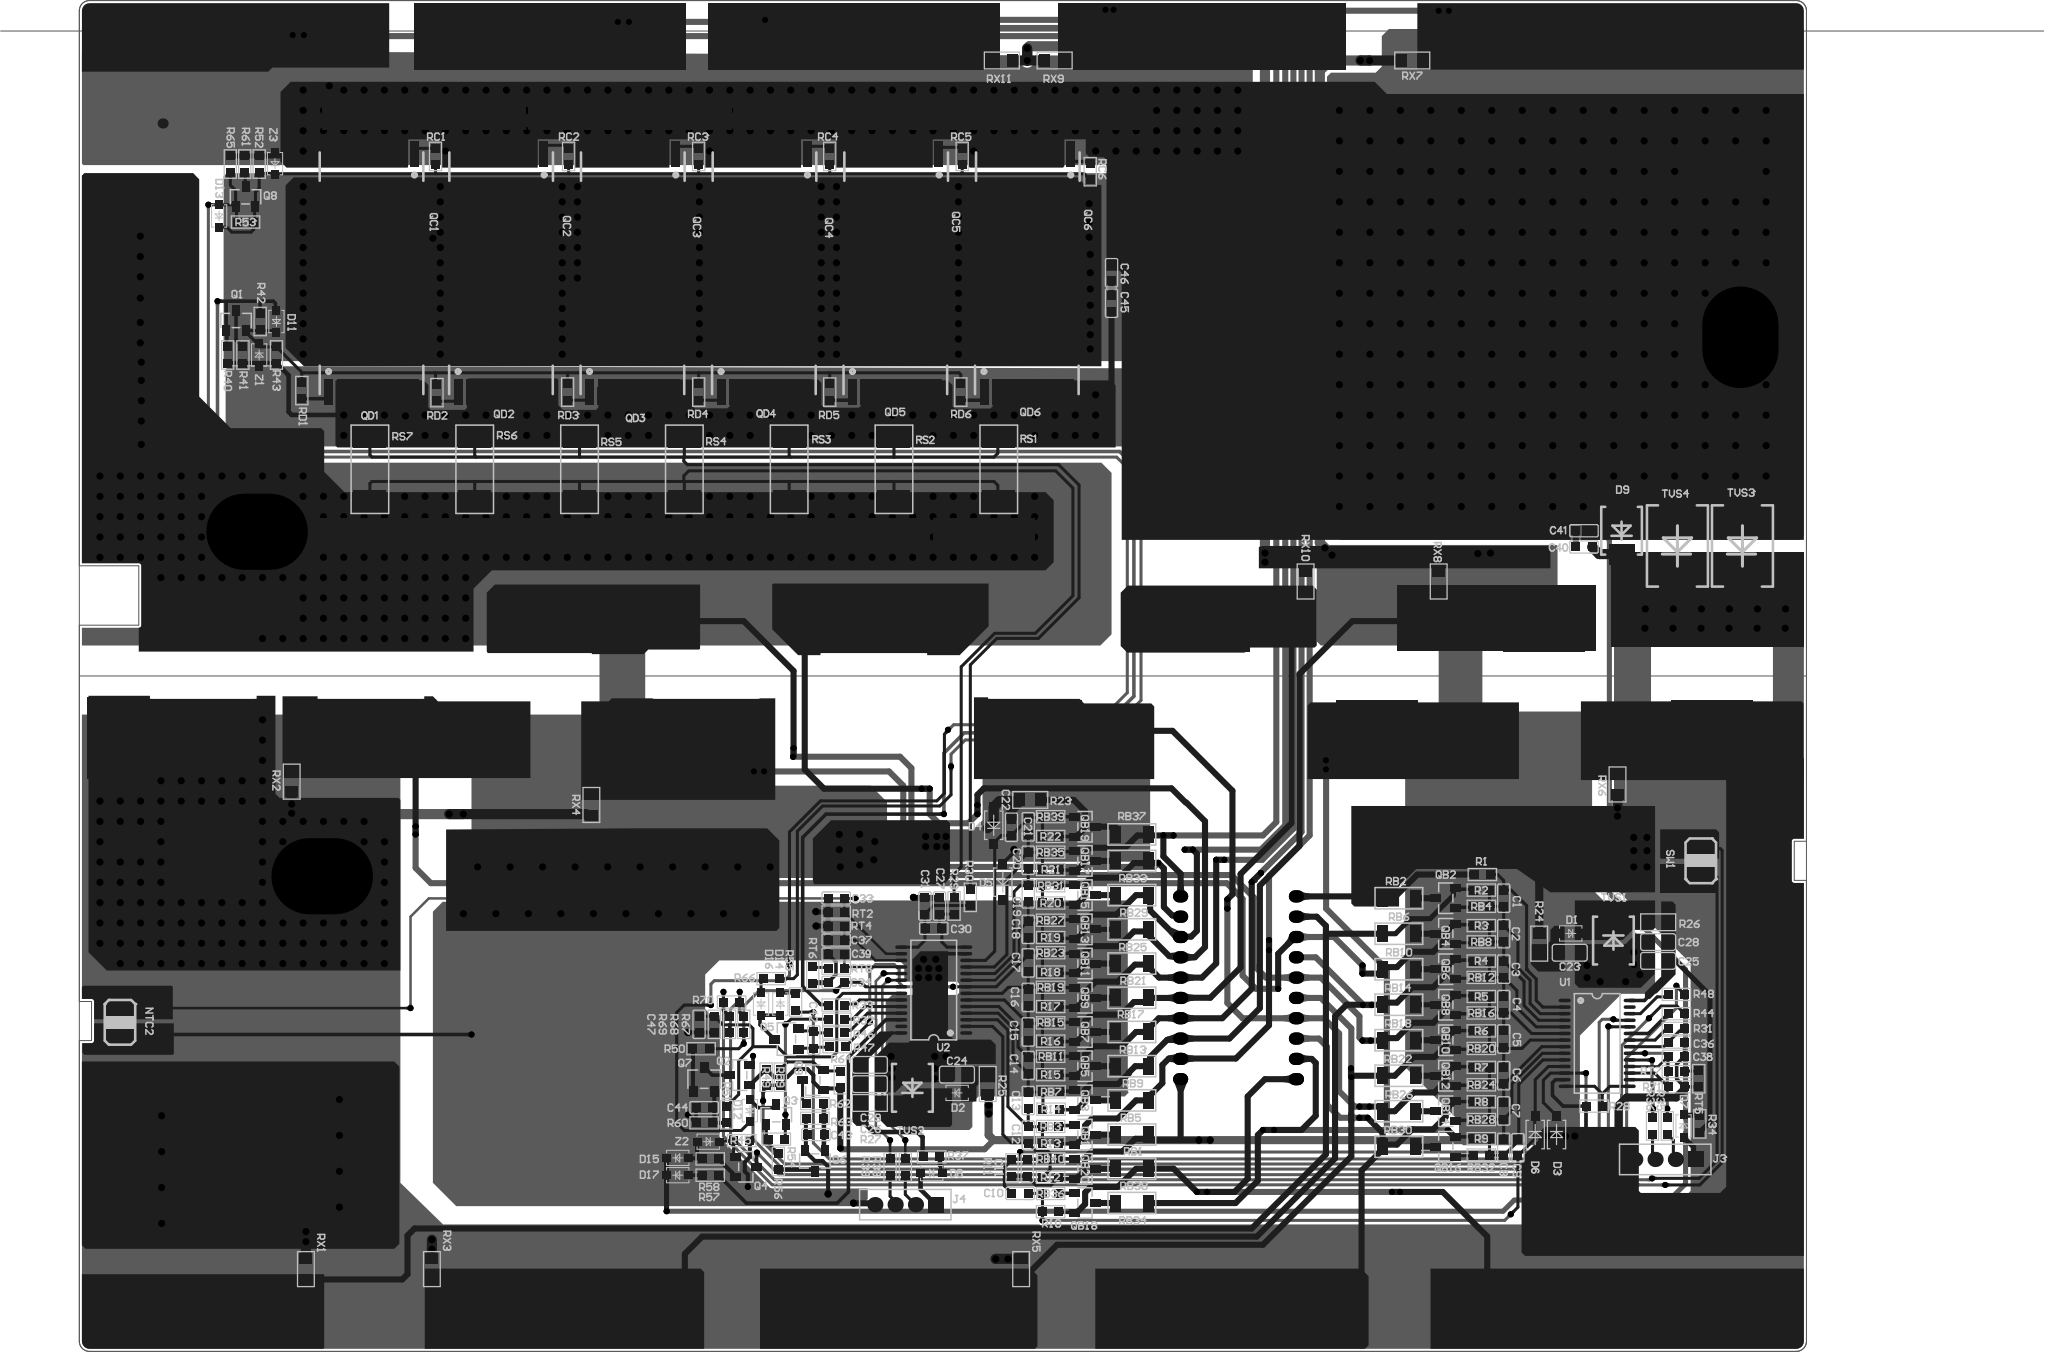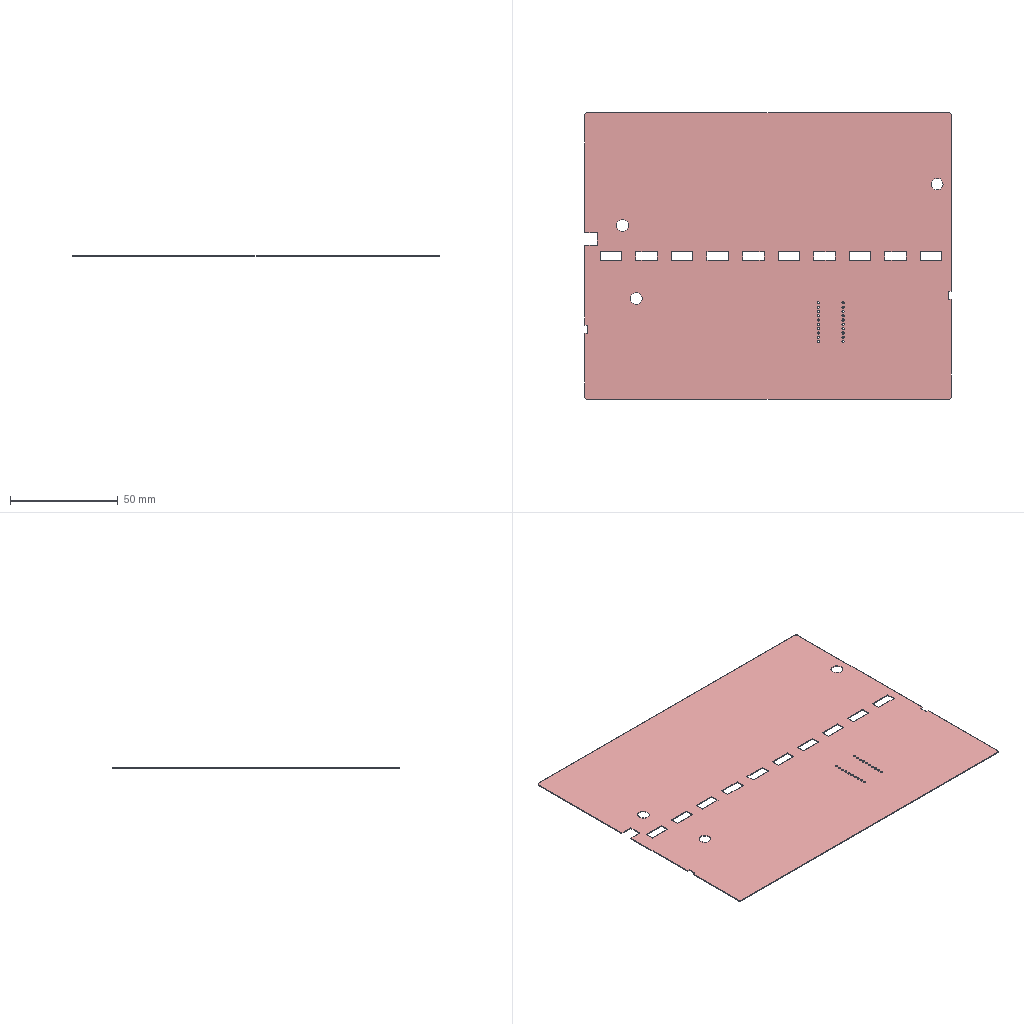Circuit board layout | Altium Designer | box 170 x 133 x 0.4 mm
Layer stack:
# Altium Designer layer stack of  (unit mm; dielectric type: 0 none, 1 core, 2 prepreg, 3 surface material)
index,name,kind,layer,copper_thickness_mm,dielectric_type,dielectric_thickness_mm,dielectric_material,dielectric_constant
0,Top Paste,other,,,,,,
1,Top Overlay,other,,,,,,
2,Top Solder,dielectric,,,3,0.0102,Solder Resist,3.5
3,Top Layer,copper,Top Layer,0.0356,,,,
4,Dielectric 1,dielectric,,,0,0.32,FR-4,4.8
5,Bottom Layer,copper,Bottom Layer,0.0356,,,,
6,Bottom Solder,dielectric,,,3,0.0102,Solder Resist,3.5
7,Bottom Overlay,other,,,,,,
8,Bottom Paste,other,,,,,,
# drill layer pairs: low layer,high layer
drill_pair,Top Layer,Bottom Layer
Part placement:
Designator,Comment,Layer,Footprint,Center-X(mm),Center-Y(mm),Rotation
RS7,R010,TopLayer,R2512L,28.6,85.85,90
RS6,R010,TopLayer,R2512L,38.917,85.85,90
RD6,47R,TopLayer,R0603A,86.76,93.45,90
RD5,47R,TopLayer,R0603A,73.86,93.45,90
RC6,47R,TopLayer,R0603A,99.5,115.15,90
RC5,47R,TopLayer,R0603A,86.9,116.65,90
QD6,N MOS*,TopLayer,TOLL_123,93.26,96.8,0
QD5,N MOS*,TopLayer,TOLL_123,80.32,96.8,0
QC6,N MOS*,TopLayer,TOLL_123,93.36,113.5,180
QC5,N MOS*,TopLayer,TOLL_123,80.4,113.5,180
R71,10K,TopLayer,R0603A,157.2,25.05,180
R70,100K,TopLayer,R0603A,64.2,33.4,0
R69,10M,TopLayer,R0603A,62.5,31.2,270
R68,100K,TopLayer,R0603A,64,31.2,90
R67,100K,TopLayer,R0603A,65.4,31.2,270
C47,1nF25V,TopLayer,C0603A,61,31.2,90
SW1,SW_1,TopLayer,RT2.3X1.2-2,159.6,47.3,90
TVS4,SMBJ75A*,TopLayer,SMC_MDO-214AB),157.3,78.3,270
TVS3,SMBJ75A*,TopLayer,SMC_MDO-214AB),163.7,78.3,270
RB40,510R,TopLayer,R0603A,95.6,17.95,180
RB39,510R,TopLayer,R0603A,95.6,51.65,180
RB38,100R,TopLayer,R1206A,103.6,16.977,180
RB37,100R,TopLayer,R1206A,103.6,49.9,180
RB36,510R,TopLayer,R0603A,95.6,14.55,180
RB35,510R,TopLayer,R0603A,95.6,48.15,180
RB34,100R,TopLayer,R1206A,103.6,13.609,180
RB33,100R,TopLayer,R1206A,103.6,47.291,180
RB32,510R,TopLayer,R0603A,138,18.332,0
RB31,510R,TopLayer,R0603A,95.6,44.85,180
RB30,100R,TopLayer,R1206A,129.884,19.15,0
RB29,100R,TopLayer,R1206A,103.6,43.923,180
RB28,510R,TopLayer,R0603A,138,21.83,0
RB27,510R,TopLayer,R0603A,95.6,41.45,180
RB26,100R,TopLayer,R1206A,129.884,22.645,0
RB25,100R,TopLayer,R1206A,103.6,40.555,180
RB24,510R,TopLayer,R0603A,138,25.25,0
RB23,510R,TopLayer,R0603A,95.6,38.25,180
RB22,100R,TopLayer,R1206A,129.884,26.141,0
RB21,100R,TopLayer,R1206A,103.6,37.186,180
RB20,510R,TopLayer,R0603A,138,28.826,0
RB19,510R,TopLayer,R0603A,95.6,34.85,180
RB18,100R,TopLayer,R1206A,129.884,29.636,0
RB17,100R,TopLayer,R1206A,103.6,33.818,180
RB16,510R,TopLayer,R0603A,138,32.324,0
RB15,510R,TopLayer,R0603A,95.6,31.35,180
RB14,100R,TopLayer,R1206A,129.884,33.131,0
RB13,100R,TopLayer,R1206A,103.6,30.45,180
RB12,510R,TopLayer,R0603A,138,35.822,0
RB11,510R,TopLayer,R0603A,95.6,28.05,180
RB10,100R,TopLayer,R1206A,129.884,36.627,0
RB9,100R,TopLayer,R1206A,103.6,27.082,180
RB8,510R,TopLayer,R0603A,138,39.32,0
RB7,510R,TopLayer,R0603A,95.65,24.55,180
RB6,100R,TopLayer,R1206A,129.884,40.122,0
RB5,100R,TopLayer,R1206A,103.6,23.714,180
RB4,510R,TopLayer,R0603A,138,42.818,0
RB3,510R,TopLayer,R0603A,95.6,21.15,180
RB2,100R,TopLayer,R1206A,129.884,43.617,0
RB1,100R,TopLayer,R1206A,103.6,20.346,180
QB20,MMBT5551,TopLayer,SOT23-3,98.992,16.977,270
QB19,MMBT5551,TopLayer,SOT23-3,98.992,50.659,270
QB18,MMBT5551,TopLayer,SOT23-3,98.992,13.609,270
QB17,MMBT5551,TopLayer,SOT23-3,98.992,47.291,270
QB16,MMBT5551,TopLayer,SOT23-3,134.492,19.15,90
QB15,MMBT5551,TopLayer,SOT23-3,98.992,43.923,270
QB14,MMBT5551,TopLayer,SOT23-3,134.492,22.645,90
QB13,MMBT5551,TopLayer,SOT23-3,98.992,40.555,270
QB12,MMBT5551,TopLayer,SOT23-3,134.492,26.141,90
QB11,MMBT5551,TopLayer,SOT23-3,98.992,37.186,270
QB10,MMBT5551,TopLayer,SOT23-3,134.492,29.636,90
QB9,MMBT5551,TopLayer,SOT23-3,98.992,33.818,270
QB8,MMBT5551,TopLayer,SOT23-3,134.492,33.131,90
QB7,MMBT5551,TopLayer,SOT23-3,98.992,30.45,270
QB6,MMBT5551,TopLayer,SOT23-3,134.492,36.627,90
QB5,MMBT5551,TopLayer,SOT23-3,98.992,27.082,270
QB4,MMBT5551,TopLayer,SOT23-3,134.492,40.122,90
QB3,MMBT5551,TopLayer,SOT23-3,98.992,23.714,270
QB2,MMBT5551,TopLayer,SOT23-3,134.492,43.617,90
QB1,MMBT5551,TopLayer,SOT23-3,98.992,20.346,270
R49,1M,TopLayer,R0603A,67.6,26,90
NTC2,10K B=3435,TopLayer,RT2.3X1.2-2,4,31.4,270
C46,0.1uF100V,TopLayer,C0603A,101.6,105.2,270
C45,0.1uF100V,TopLayer,C0603A,101.6,102.2,270
D7,BAV21W,TopLayer,SOD323A,157.9,21.2,270
RX11,0R,TopLayer,R0805L,90.8,126.1,180
RX3,0R,TopLayer,R0805L,34.7,7.1,270
Q9,MMBT5401,TopLayer,SOT23-3,72.192,25.7,90
R64,1M,TopLayer,R0603A,74.9,25.75,270
Q8,MMBT5401,TopLayer,SOT23-3,16.36,112.684,0
R36,100R,TopLayer,R0603A,154.85,21.2,270
R35,100R,TopLayer,R0603A,156.3,21.2,270
R38,100R,TopLayer,R0603A,81.3,17.15,270
R37,100R,TopLayer,R0603A,83.9,18.15,0
RD4,47R,TopLayer,R0603A,60.96,93.45,90
RD3,47R,TopLayer,R0603A,48.06,93.45,270
RD2,47R,TopLayer,R0603A,35.2,93.4,270
TVS2,SMBJ64A,TopLayer,SMB_A,82,24.95,90
TVS1,SMBJ64A,TopLayer,SMB_A,151,39.45,270
D4,BAT46W,TopLayer,SOD123,90,50.8,90
D3,BAT46W,TopLayer,SOD123,145.4,20.35,270
R61,510R,TopLayer,R0603A,16.28,115.9,90
R33,1K,TopLayer,R0603A,74.5,33.1,180
C26,1uF100V,TopLayer,C0805L,77.81,25.31,180
C25,1uF100V,TopLayer,C0805L,155.4,37.45,0
C24,1uF100V,TopLayer,C0805L,86.384,26.25,0
C23,1uF100V,TopLayer,C0805L,146.7,38.25,180
C22,1uF50V,TopLayer,C0603A,91.75,50.6,270
C21,0.1uF50V,TopLayer,C0603A,93.4,50.65,270
C20,0.1uF50V,TopLayer,C0603A,93.4,47.35,270
C19,0.1uF50V,TopLayer,C0603A,93.4,44.05,270
C17,0.1uF50V,TopLayer,C0603A,93.4,37.25,270
C16,0.1uF50V,TopLayer,C0603A,93.4,33.85,270
C15,0.1uF50V,TopLayer,C0603A,93.4,30.45,270
C14,0.1uF50V,TopLayer,C0603A,93.4,27.15,270
C13,0.1uF50V,TopLayer,C0603A,93.4,23.7,270
C12,0.1uF50V,TopLayer,C0603A,93.4,20.3,270
C8,0.1uF50V,TopLayer,C0603A,140.2,19.082,90
C7,0.1uF50V,TopLayer,C0603A,140.2,22.673,90
C6,0.1uF50V,TopLayer,C0603A,140.2,26.15,90
C5,0.1uF50V,TopLayer,C0603A,140.2,29.755,90
C4,0.1uF50V,TopLayer,C0603A,140.2,33.145,90
C3,0.1uF50V,TopLayer,C0603A,140.2,36.636,90
C1,0.1uF50V,TopLayer,C0603A,140.2,43.617,90
RT2,10K B=3435,TopLayer,R0603A,74.5,42.26,180
R66,1M,TopLayer,R0603A,68.1,35.7,180
R65,5.1M,TopLayer,R0603A,14.86,115.9,90
R63,1M,TopLayer,R0603A,72.4,21.95,180
R62,3M,TopLayer,R0603A,72.4,23.4,180
R59,3M,TopLayer,R0603A,69,26,270
R58,1M,TopLayer,R0603A,62.1,17.95,0
R57,3M,TopLayer,R0603A,62.1,16.35,0
R56,3M,TopLayer,R0603A,68.8,17.7,270
R55,1M,TopLayer,R0603A,70.5,33.4,270
R54,1M,TopLayer,R0603A,68.6,19.9,0
R53,0R/NC*,TopLayer,R0603A,16.36,110.192,0
R52,5.1M,TopLayer,R0603A,17.7,115.9,90
R51,100K,TopLayer,R0603A,63.7,22.3,90
R50,100K,TopLayer,R0603A,61.2,28.8,0
RC1,47R,TopLayer,R0603A,35.06,116.65,90
R48,10M,TopLayer,R0603A,157.2,34.15,180
R47,10K,TopLayer,R0603A,74.6,29,0
R46,10K,TopLayer,R0603A,74.56,30.36,0
R45,510K,TopLayer,R0603A,65.2,19.75,180
R44,1M,TopLayer,R0603A,157.2,32.25,180
R43,5.1M,TopLayer,R0603A,19.4,97.1,270
R42,0R/NC*,TopLayer,R0603A,17.8,100.4,270
R41,510R,TopLayer,R0603A,16.1,97.1,270
R40,5.1M,TopLayer,R0603A,14.6,97.1,270
R39,100R,TopLayer,R0603A,79.8,17.15,270
R34,100R,TopLayer,R0603A,159.5,21.4,90
R32,1K,TopLayer,R0603A,74.56,31.71,180
R31,1K,TopLayer,R0603A,157.2,30.8,180
R30,10R,TopLayer,R0603A,87.7,43.7,90
R29,10R,TopLayer,R0603A,86.1,42.85,270
R28,1K,TopLayer,R0603A,149.1,23.15,0
R27,100R,TopLayer,R0805L,77.81,23.46,0
R26,100R,TopLayer,R0805L,155.4,41.25,180
R25,1K,TopLayer,R0805L,89.41,25.326,270
R20,510R,TopLayer,R0603A,95.6,43.15,180
R19,510R,TopLayer,R0603A,95.6,39.75,180
R18,510R,TopLayer,R0603A,95.6,36.35,180
R17,510R,TopLayer,R0603A,95.6,32.95,180
R16,510R,TopLayer,R0603A,95.6,29.55,180
R15,510R,TopLayer,R0603A,95.6,26.25,180
R14,510R,TopLayer,R0603A,95.65,22.85,180
R13,510R,TopLayer,R0603A,95.6,19.5,180
R12,510R,TopLayer,R0603A,95.6,16.15,180
R11,510R,TopLayer,R0603A,91.8,17.05,90
R10,510R,TopLayer,R0603A,95.6,12.75,180
R8,510R,TopLayer,R0603A,138,23.573,0
R7,510R,TopLayer,R0603A,138,26.964,0
R6,510R,TopLayer,R0603A,138,30.555,0
R5,510R,TopLayer,R0603A,138,33.945,0
R4,510R,TopLayer,R0603A,138,37.436,0
R3,510R,TopLayer,R0603A,138,40.927,0
R1,510R,TopLayer,R0603A,138.1,45.95,0
Q5,AM2394,TopLayer,SOT23-3L,69.6,29.75,90
Q2,MMBT5401,TopLayer,SOT23-3,64.992,26.2,90
Q1,MMBT5401,TopLayer,SOT23-3,15.425,100.508,0
D11,BAV21W,TopLayer,SOD323A,19.4,100.4,90
D9,RS3M,TopLayer,SMB_A,151.8,79.8,90
D2,BAV21W,TopLayer,SOD323A,86.4,24.45,0
D1,BAV21W,TopLayer,SOD323A,146.8,40.15,180
C44,1nF25V,TopLayer,C0603A,61.5,23,180
C37,1nF25V,TopLayer,C0603A,74.5,39.5,180
C36,1uF25V,TopLayer,C0603A,157.2,29.45,180
C34,1uF25V,TopLayer,C0603A,74.5,35.34,0
C33,1nF25V,TopLayer,C0603A,74.5,43.64,180
C31,1uF25V,TopLayer,C0603A,83.233,42.85,270
C30,1nF25V,TopLayer,C0603A,84.1,40.65,0
C29,0.1uF100V,TopLayer,C0805L,77.81,27.21,180
C28,0.1uF100V,TopLayer,C0805L,155.4,39.3,0
C27,1uF25V,TopLayer,C0603A,84.667,42.85,90
C18,0.1uF50V,TopLayer,C0603A,93.4,40.55,270
C11,1uF50V,TopLayer,C0603A,93.3,17.05,90
C10,0.1uF50V,TopLayer,C0603A,92.6,14.55,0
QC4,N MOS*,TopLayer,TOLL_123,67.44,113.5,180
QC3,N MOS*,TopLayer,TOLL_123,54.48,113.5,180
Z3,15V,TopLayer,SOD323A,19.26,115.942,90
Z2,3.3V,TopLayer,SOD323A,61.9,19.65,180
Z1,15V,TopLayer,SOD323A,17.7,97.1,270
RX10,0R,TopLayer,R0805L,120.7,74.8,270
RX9,0R,TopLayer,R0805L,96,126.1,0
RX8,0R,TopLayer,R0805L,133.8,74.8,270
RX7,0R,TopLayer,R0805L,131.2,126.1,0
RX6,0R,TopLayer,R0805L,151.4,54.816,270
RX5,0R,TopLayer,R0805L,92.7,7.1,270
RX4,0R,TopLayer,R0805L,50.4,52.8,90
RX2,0R,TopLayer,R0805L,20.9,55.1,90
RX1,0R,TopLayer,R0805L,22.3,7.1,270
RT8,0R,TopLayer,R0603A,74.5,36.74,0
RT7,0R,TopLayer,R0603A,157.2,26.55,180
RT6,10K B=3435,TopLayer,R0603A,72.19,36.07,270
RT5,10K B=3435,TopLayer,R0603A,159.4,25.85,270
RT4,10K B=3435,TopLayer,R0603A,74.5,40.88,180
RS5,R010,TopLayer,R2512L,49.233,85.85,90
RS4,R010,TopLayer,R2512L,59.55,85.85,90
RD1,47R,TopLayer,R0603A,21.9,93.6,270
RC4,47R,TopLayer,R0603A,73.86,116.65,90
RC3,47R,TopLayer,R0603A,60.96,116.65,270
RC2,47R,TopLayer,R0603A,48.16,116.65,270
R60,10M,TopLayer,R0603A,61.5,21.5,0
R24,1K,TopLayer,R0805L,143.7,39.15,90
R23,510R,TopLayer,R0805L,93.6,53.3,0
R22,510R,TopLayer,R0603A,95.6,49.7,180
R21,510R,TopLayer,R0603A,95.6,46.45,180
R9,510R,TopLayer,R0603A,138,19.95,0
R2,510R,TopLayer,R0603A,138,44.417,0
QC2,N MOS*,TopLayer,TOLL_123,41.52,113.5,180
QC1,N MOS*,TopLayer,TOLL_123,28.76,113.5,180
QD2,N MOS*,TopLayer,TOLL_123,41.5,96.8,0
Q7,AM2394,TopLayer,SOT23-3L,61.5,25.8,0
Q6,MMBT5551,TopLayer,SOT23-3,72.4,17.742,180
Q4,MMBT5551,TopLayer,SOT23-3,65.608,17.175,270
Q3,MMBT5401,TopLayer,SOT23-3,68.6,22.308,0
J4,CH-2.0-4P,TopLayer,Test2.0-4P,81.3,13.45,180
J3,CH-2.0-4P,TopLayer,Test2.0-4P,156.1,17.9,180
D17,BAV21W,TopLayer,SOD323A,58.9,16.35,0
D16,BAV21W,TopLayer,SOD323A,67.1,33.2,90
D15,BAV21W,TopLayer,SOD323A,58.9,18.05,0
D14,BAV21W,TopLayer,SOD323A,69,33.2,270
D13,BAV21W,TopLayer,SOD323A,13.76,110.792,90
D12,BAV21W,TopLayer,SOD323A,66,22.7,90
C43,0.1uF50V,TopLayer,C0603A,72.5,20.35,0
C42,10nF25V,TopLayer,C0603A,72.3,29.65,90
C9,0.1uF50V,TopLayer,C0603A,141.6,19.05,90
C2,0.1uF50V,TopLayer,C0603A,140.2,40.127,90
D6,BAT46W,TopLayer,SOD123,143.3,20.35,270
C38,1nF25V,TopLayer,C0603A,157.2,28.05,0
RS3,R010,TopLayer,R2512L,69.867,85.85,90
QD4,N MOS*,TopLayer,TOLL_123,67.38,96.8,0
U2,SH3676010,TopLayer,TSSOP-28L(PIN间距0.65mm),84.1,34.575,180
U1,SH3676010,TopLayer,TSSOP-28L(PIN间距0.65mm),149.4,29.325,0
RS2,R010,TopLayer,R2512L,80.183,85.85,90
RS1,R010,TopLayer,R2512L,90.5,85.85,90
QD3,N MOS*,TopLayer,TOLL_123,54.44,96.8,0
D8,BAV21W,TopLayer,SOD323A,83.9,16.55,180
D5,BAT46W,TopLayer,SOD123,90.9,45.2,90
C41,0.1uF50V,TopLayer,C0603A,148.1,79.8,180
C39,1nF25V,TopLayer,C0603A,74.5,38.12,180
C40,0.1uF50V,TopLayer,C0603A,148.1,78.2,0
QD1,N MOS*,TopLayer,TOLL_123,28.76,96.8,0
Pad and via stacks:
# Altium Designer via and pad stacks of  (unit mm). Each distinct definition once, with the count of objects using it.
# via: kind,start_layer,end_layer,hole_mm,diameter_mm,mode(0 simple;1 top-mid-bottom;2 full stack),diameter_per_layer,count,example_net
# pad: kind,layer,hole_mm,hole_type(0 round;1 square;2 slot),plating,top_size,top_shape(1 round;2 rect;3 octagon;9 rounded rect),mid_size,bottom_size,mode,footprint,size_per_layer,count,example
pad,Top Layer,0,0,plated,8x6,2,8x6,8x6,0,,,21,81
pad,Top Layer,0,0,plated,3x3,1,3x3,3x3,0,,,23,86
pad,Top Layer,0,0,plated,2.5x20,2,2.5x20,2.5x20,0,,,7,82
pad,Top Layer,0,0,plated,2.5x10,2,2.5x10,2.5x10,0,,,1,83
pad,Top Layer,0,0,plated,0.8x0.8,2,0.8x0.8,0.8x0.8,0,R0603A,,208,R9.1
pad,Top Layer,0,0,plated,0.8x0.8,2,0.8x0.8,0.8x0.8,0,C0603A,,78,C9.1
pad,Top Layer,0,0,plated,0.9x0.8,2,0.9x0.8,0.9x0.8,0,SOD123,,8,D6.2
pad,Top Layer,0,0,plated,1.016x1.27,2,1.016x1.27,1.016x1.27,0,R0805L,,32,R24.1
pad,Top Layer,0,0,plated,1.5x1.5,2,1.5x1.5,1.5x1.5,0,Test2.0-4P,,2,J3.1
pad,Top Layer,0,0,plated,1.5x1.5,1,1.5x1.5,1.5x1.5,0,Test2.0-4P,,6,J3.2
pad,Top Layer,0,2,plated,1.2x0.35,1,1.2x0.35,1.2x0.35,0,TSSOP-28L(PIN\u00BC\u00E4\u00BE\u00E00.65mm),,56,U1.1
pad,Top Layer,0,0,plated,0.7x1,2,0.7x1,0.7x1,0,SOT23-3,,81,QB16.1
pad,Top Layer,0,0,plated,1x1.6,2,1x1.6,1x1.6,0,R1206A,,40,RB10.1
pad,Top Layer,0,0,plated,1.016x1.27,2,1.016x1.27,1.016x1.27,0,C0805L,,12,C23.2
pad,Top Layer,0,0,plated,0.8x0.7,2,0.8x0.7,0.8x0.7,0,SOD323A,,28,D1.1
pad,Top Layer,0,0,plated,2x2.5,2,2x2.5,2x2.5,0,SMB A,,6,TVS1.1
pad,Top Layer,0,0,plated,0.8x1,2,0.8x1,0.8x1,0,SOT23-3L,,6,Q7.1
pad,Top Layer,0,0,plated,2.5x0.8,2,2.5x0.8,2.5x0.8,0,TOLL_123,,12,QC3.1
pad,Top Layer,0,0,plated,1.7x0.8,2,1.7x0.8,1.7x0.8,0,TOLL_123,,84,QC3.2
pad,Top Layer,0,0,plated,0.8x8,2,0.8x8,0.8x8,0,TOLL_123,,12,QC3.2
pad,Top Layer,0,0,plated,9.9x8,2,9.9x8,9.9x8,0,TOLL_123,,12,QC3.3
pad,Top Layer,0,0,plated,2x3.2,2,2x3.2,2x3.2,0,R2512L,,14,RS6.2
pad,Top Layer,0,0,plated,1.8x3.2,2,1.8x3.2,1.8x3.2,0,SMC_MDO-214AB),,4,TVS3.2
pad,Top Layer,0,0,plated,9x6,2,9x6,9x6,0,,,1,81
pad,Top Layer,0,0,plated,1.2x2.3,1,1.2x2.3,1.2x2.3,0,RT2.3X1.2-2,,4,SW1.1
pad,Top Layer,0,0,plated,1x1,1,1x1,1x1,0,,,2,75
pad,Multi-Layer,1,0,plated,1.5x1.2,1,1.5x1.2,1.5x1.2,0,,,20,
pad,Multi-Layer,5.5,0,plated,7.5x10,1,7.5x10,7.5x10,0,,,3,66
via,Top Layer,Bottom Layer,0.4,0.6,0,,99,B15
via,Top Layer,Bottom Layer,0.5,0.7,0,,953,GND
Copper pours:
name,layer,net,type(0 solid;1 hatched;2 none)
NONET_L02_P-001,Top Layer,NetR68_2,0
NONET_L02_P-001,Top Layer,NetR67_1,0
NONET_L02_P-001,Top Layer,P-/C-,0
NONET_L02_P-001,Top Layer,B4,0
NONET_L02_P-001,Top Layer,B14,0
NONET_L02_P-001,Top Layer,B13,0
NONET_L02_P-001,Top Layer,B+,0
NONET_L02_P-001,Top Layer,B17,0
NONET_L02_P-001,Top Layer,B+,0
NONET_L02_P-001,Top Layer,B10,0
NONET_L02_P-001,Top Layer,GND,0
NONET_L02_P-001,Top Layer,B12,0
NONET_L02_P-001,Top Layer,NetC33_1,0
NONET_L02_P-001,Top Layer,GND,0
NONET_L02_P-001,Top Layer,GND,0
NONET_L02_P-001,Top Layer,B10,0
NONET_L02_P-001,Top Layer,VBAT_S,0
NONET_L02_P-001,Top Layer,B10,0
NONET_L02_P-001,Top Layer,NetD1_1,0
NONET_L02_P-001,Top Layer,NetC23_2,0
NONET_L02_P-001,Top Layer,B6,0
NONET_L02_P-001,Top Layer,VBAT_M,0
NONET_L02_P-001,Top Layer,NetC24_2,0
NONET_L02_P-001,Top Layer,GND,0
NONET_L02_P-001,Top Layer,NetD2_1,0
NONET_L02_P-001,Top Layer,GND,0
NONET_L02_P-001,Top Layer,NetC45_2,0
NONET_L02_P-001,Top Layer,B+,0
NONET_L02_P-001,Top Layer,B9,0
NONET_L02_P-001,Top Layer,B+,0
NONET_L02_P-001,Top Layer,B8,0
NONET_L02_P-001,Top Layer,B10,0
NONET_L02_P-001,Top Layer,B16,0
NONET_L02_P-001,Top Layer,B2,0
NONET_L02_P-001,Top Layer,B18,0
NONET_L02_P-001,Top Layer,B11,0
NONET_L02_P-001,Top Layer,B15,0
NONET_L02_P-001,Top Layer,B19,0
NONET_L02_P-001,Top Layer,B7,0
NONET_L02_P-001,Top Layer,B5,0
NONET_L02_P-001,Top Layer,B3,0
NONET_L02_P-001,Top Layer,B1,0
NONET_L02_P-001,Top Layer,MSO_D-,0
NONET_L02_P-001,Bottom Layer,GND,0
NONET_L02_P-001,Bottom Layer,B+,0
NONET_L02_P-001,Bottom Layer,GND,0
NONET_L02_P-001,Bottom Layer,GND,0
NONET_L02_P-001,Bottom Layer,B10,0
NONET_L02_P-001,Bottom Layer,P-/C-,0
NONET_L02_P-001,Bottom Layer,P-/C-,0
NONET_L02_P-001,Bottom Layer,MSO_D-,0
NONET_L02_P-001,Bottom Layer,NetC45_2,0
NONET_L02_P-001,Bottom Layer,GND,0
Design rules, without the lines most boards share:
# Altium Designer design rules of  (exported by Altium Designer, unit mm)
# columns: name | kind | enabled | priority | scope1 | scope2 | descriptor | typed fields (field=value)
Schematic Supply Nets_3 | 41 | enabled | 1 | InNet('B0') | All | Supply Net(s)(InNet('B0')) |
Schematic Supply Nets_2 | 41 | enabled | 2 | InNet('P-/C-') | All | Supply Net(s)(InNet('P-/C-')) |
Schematic Supply Nets_1 | 41 | enabled | 3 | InNet('GND') | All | Supply Net(s)(InNet('GND')) |
Schematic Supply Nets | 41 | enabled | 4 | InNet('B10') | All | Supply Net(s)(InNet('B10')) |
NetAntennae | 56 | enabled | 1 | All | All | Net Antennae (Tolerance=0mm) (All) |
SilkToSilkClearance | 55 | enabled | 1 | All | All | Silk to Silk (Clearance=0.254mm) (All),(All) |
SilkToSolderMaskClearance | 54 | enabled | 1 | IsPad | All | Silk To Solder Mask (Clearance=0.254mm) (IsPad),(All) |
MinimumSolderMaskSliver | 53 | enabled | 1 | All | All | Minimum Solder Mask Sliver (Gap=0.254mm) (All),(All) |
HoleToHoleClearance | 52 | enabled | 1 | All | All | Hole To Hole Clearance (Gap=0.254mm) (All),(All) | gap=0.254
DiffPairsRouting | 51 | enabled | 1 | All | All | Differential Pairs Uncoupled Length using the Gap Constraints (Min=0.254mm) (Max=0.254mm) (Prefered=0.254mm)  and Width Constraints (Min=0.381mm) (Max=0.381mm) (Prefered=0.381mm) (All) |
HoleSize | 42 | enabled | 1 | All | All | Hole Size Constraint (Min=0.025mm) (Max=50mm) (All) |
Height | 50 | enabled | 1 | All | All | Height Constraint (Min=0mm) (Max=25.4mm) (Prefered=12.7mm) (All) | min_height=0 max_height=25.4
ComponentClearance | 24 | enabled | 1 | All | All | Component Clearance Constraint ( Horizontal Gap = 0.2mm, Vertical Gap = 0.2mm ) (All),(All)  | gap=0.2
SolderMaskExpansion | 13 | enabled | 1 | All | All | Solder Mask Expansion (Expansion =0.102mm) (All) | expansion=0.1016
PasteMaskExpansion | 14 | enabled | 1 | All | All | Paste Mask Expansion (Expansion =0mm) (All) | expansion=0
RoutingVias | 11 | enabled | 1 | All | All | Routing Via (MinHoleWidth=0.4mm) (MaxHoleWidth=0.5mm) (PreferredHoleWidth=0.4mm) (MinWidth=0.6mm) (MaxWidth=7mm) (PreferedWidth=0.6mm) (All) | via_min_hole=0.4 via_max_hole=0.5 via_preferred_diameter=0.6 via_preferred_hole=0.4
RoutingCorners | 10 | enabled | 1 | All | All | Routing Corners (Style=45-Degree) (Min Setback=2.54mm) (Max Setback=2.54mm) (All) |
Width | 2 | enabled | 1 | All | All | Width Constraint (Min=0.2mm) (Max=2mm) (Preferred=0.25mm) (All) |
PolygonConnect | 20 | enabled | 1 | All | All | Polygon Connect Rule(Direct Connect )(Conductor Width=0.254mm) (Relief Angle=90 Angle) (Entries=4) (Air Gap Width=0.254mm) (All),(All) | connect_style(0=relief,1=direct,2=none)=1 relief_conductor_width=0.254 relief_entries=4
PlaneClearance | 12 | enabled | 1 | All | All | Power Plane Clearance (Clearance =0.508mm) (All) | clearance=0.508
PlaneConnect | 6 | enabled | 1 | All | All | Power Plane Connect Rule(Relief Connect )(Expansion=0.508mm) (Conductor Width=0.254mm) (Air Gap=0.254mm) (Entries=4) (All) | relief_conductor_width=0.254 relief_entries=4 relief_expansion=0.508
Clearance | 0 | enabled | 1 | All | All | Clearance Constraint (Gap=0.2mm) (All),(All) | gap=0.2